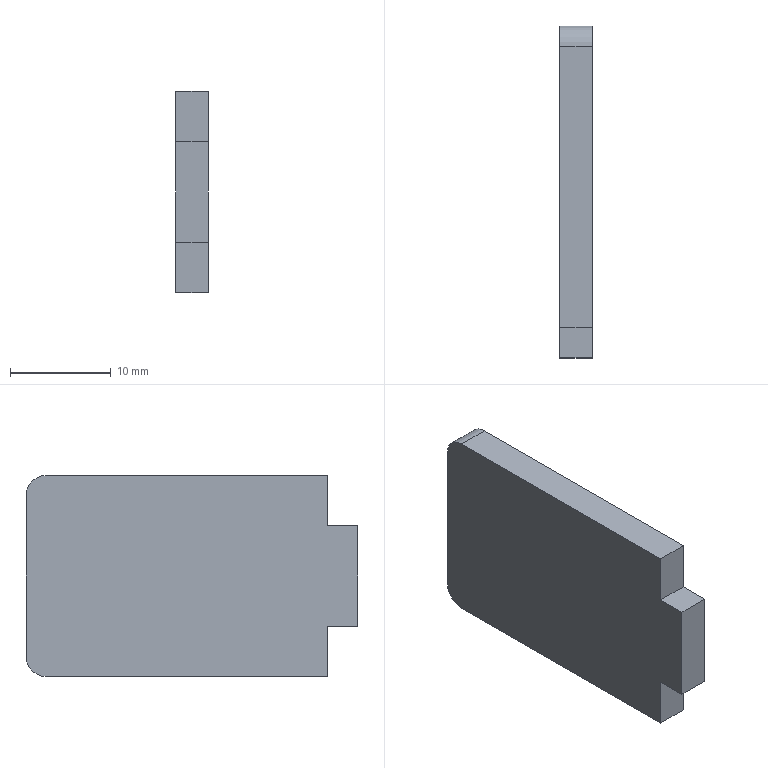Part | SolidWorks | features FlatPattern 1, SMBaseFlange 1, SheetMetal 1 | 1 solid | 12 faces | box 3.2 x 33 x 20 mm | volume 2011 mm3 | plane 10 | cylinder 2 | commonest cylinder face diameters 4 x2
STEP:
#1=CARTESIAN_POINT('',(0.,-30.,0.));
#2=VERTEX_POINT('',#1);
#3=CARTESIAN_POINT('',(0.,-30.,-5.));
#4=VERTEX_POINT('',#3);
#5=CARTESIAN_POINT('',(0.,-30.,0.));
#6=DIRECTION('',(0.,0.,-1.));
#7=VECTOR('',#6,1000.);
#8=LINE('',#5,#7);
#9=EDGE_CURVE('',#2,#4,#8,.T.);
#10=ORIENTED_EDGE('',*,*,#9,.F.);
#11=CARTESIAN_POINT('',(-3.2,-30.,0.));
#12=VERTEX_POINT('',#11);
#13=CARTESIAN_POINT('',(-3.2,-30.,0.));
#14=DIRECTION('',(1.,0.,0.));
#15=VECTOR('',#14,1000.);
#16=LINE('',#13,#15);
#17=EDGE_CURVE('',#12,#2,#16,.T.);
#18=ORIENTED_EDGE('',*,*,#17,.F.);
#19=CARTESIAN_POINT('',(-3.2,-30.,-5.));
#20=VERTEX_POINT('',#19);
#21=CARTESIAN_POINT('',(-3.2,-30.,0.));
#22=DIRECTION('',(0.,0.,-1.));
#23=VECTOR('',#22,1000.);
#24=LINE('',#21,#23);
#25=EDGE_CURVE('',#12,#20,#24,.T.);
#26=ORIENTED_EDGE('',*,*,#25,.T.);
#27=CARTESIAN_POINT('',(-3.2,-30.,-5.));
#28=DIRECTION('',(1.,0.,0.));
#29=VECTOR('',#28,1000.);
#30=LINE('',#27,#29);
#31=EDGE_CURVE('',#20,#4,#30,.T.);
#32=ORIENTED_EDGE('',*,*,#31,.T.);
#33=EDGE_LOOP('',(#10,#18,#26,#32));
#34=FACE_OUTER_BOUND('',#33,.T.);
#35=CARTESIAN_POINT('',(-3.2,-30.,0.));
#36=DIRECTION('',(0.,-1.,0.));
#37=DIRECTION('',(0.,0.,-1.));
#38=AXIS2_PLACEMENT_3D('',#35,#36,#37);
#39=PLANE('',#38);
#40=ADVANCED_FACE('',(#34),#39,.T.);
#41=CARTESIAN_POINT('',(0.,-2.,0.));
#42=VERTEX_POINT('',#41);
#43=CARTESIAN_POINT('',(0.,-2.,0.));
#44=DIRECTION('',(0.,-1.,0.));
#45=VECTOR('',#44,1000.);
#46=LINE('',#43,#45);
#47=EDGE_CURVE('',#42,#2,#46,.T.);
#48=ORIENTED_EDGE('',*,*,#47,.F.);
#49=CARTESIAN_POINT('',(-3.2,-2.,0.));
#50=VERTEX_POINT('',#49);
#51=CARTESIAN_POINT('',(-3.2,-2.,0.));
#52=DIRECTION('',(1.,0.,0.));
#53=VECTOR('',#52,1000.);
#54=LINE('',#51,#53);
#55=EDGE_CURVE('',#50,#42,#54,.T.);
#56=ORIENTED_EDGE('',*,*,#55,.F.);
#57=CARTESIAN_POINT('',(-3.2,-2.,0.));
#58=DIRECTION('',(0.,-1.,0.));
#59=VECTOR('',#58,1000.);
#60=LINE('',#57,#59);
#61=EDGE_CURVE('',#50,#12,#60,.T.);
#62=ORIENTED_EDGE('',*,*,#61,.T.);
#63=ORIENTED_EDGE('',*,*,#17,.T.);
#64=EDGE_LOOP('',(#48,#56,#62,#63));
#65=FACE_OUTER_BOUND('',#64,.T.);
#66=CARTESIAN_POINT('',(-3.2,-2.,0.));
#67=DIRECTION('',(0.,0.,1.));
#68=DIRECTION('',(1.,0.,0.));
#69=AXIS2_PLACEMENT_3D('',#66,#67,#68);
#70=PLANE('',#69);
#71=ADVANCED_FACE('',(#65),#70,.T.);
#72=CARTESIAN_POINT('',(0.,0.,-2.));
#73=VERTEX_POINT('',#72);
#74=CARTESIAN_POINT('',(0.,-2.,-2.));
#75=DIRECTION('',(1.,0.,0.));
#76=DIRECTION('',(0.,0.,1.));
#77=AXIS2_PLACEMENT_3D('',#74,#75,#76);
#78=CIRCLE('',#77,2.);
#79=EDGE_CURVE('',#73,#42,#78,.T.);
#80=ORIENTED_EDGE('',*,*,#79,.F.);
#81=CARTESIAN_POINT('',(-3.2,0.,-2.));
#82=VERTEX_POINT('',#81);
#83=CARTESIAN_POINT('',(-3.2,0.,-2.));
#84=DIRECTION('',(1.,0.,0.));
#85=VECTOR('',#84,1000.);
#86=LINE('',#83,#85);
#87=EDGE_CURVE('',#82,#73,#86,.T.);
#88=ORIENTED_EDGE('',*,*,#87,.F.);
#89=CARTESIAN_POINT('',(-3.2,-2.,-2.));
#90=DIRECTION('',(1.,0.,0.));
#91=DIRECTION('',(0.,0.,1.));
#92=AXIS2_PLACEMENT_3D('',#89,#90,#91);
#93=CIRCLE('',#92,2.);
#94=EDGE_CURVE('',#82,#50,#93,.T.);
#95=ORIENTED_EDGE('',*,*,#94,.T.);
#96=ORIENTED_EDGE('',*,*,#55,.T.);
#97=EDGE_LOOP('',(#80,#88,#95,#96));
#98=FACE_OUTER_BOUND('',#97,.T.);
#99=CARTESIAN_POINT('',(-3.2,-2.,-2.));
#100=DIRECTION('',(1.,0.,0.));
#101=DIRECTION('',(0.,0.,-1.));
#102=AXIS2_PLACEMENT_3D('',#99,#100,#101);
#103=CYLINDRICAL_SURFACE('',#102,2.);
#104=ADVANCED_FACE('',(#98),#103,.T.);
#105=CARTESIAN_POINT('',(0.,0.,-18.));
#106=VERTEX_POINT('',#105);
#107=CARTESIAN_POINT('',(0.,0.,-18.));
#108=DIRECTION('',(0.,0.,1.));
#109=VECTOR('',#108,1000.);
#110=LINE('',#107,#109);
#111=EDGE_CURVE('',#106,#73,#110,.T.);
#112=ORIENTED_EDGE('',*,*,#111,.F.);
#113=CARTESIAN_POINT('',(-3.2,0.,-18.));
#114=VERTEX_POINT('',#113);
#115=CARTESIAN_POINT('',(-3.2,0.,-18.));
#116=DIRECTION('',(1.,0.,0.));
#117=VECTOR('',#116,1000.);
#118=LINE('',#115,#117);
#119=EDGE_CURVE('',#114,#106,#118,.T.);
#120=ORIENTED_EDGE('',*,*,#119,.F.);
#121=CARTESIAN_POINT('',(-3.2,0.,-18.));
#122=DIRECTION('',(0.,0.,1.));
#123=VECTOR('',#122,1000.);
#124=LINE('',#121,#123);
#125=EDGE_CURVE('',#114,#82,#124,.T.);
#126=ORIENTED_EDGE('',*,*,#125,.T.);
#127=ORIENTED_EDGE('',*,*,#87,.T.);
#128=EDGE_LOOP('',(#112,#120,#126,#127));
#129=FACE_OUTER_BOUND('',#128,.T.);
#130=CARTESIAN_POINT('',(-3.2,0.,-18.));
#131=DIRECTION('',(0.,1.,0.));
#132=DIRECTION('',(0.,0.,1.));
#133=AXIS2_PLACEMENT_3D('',#130,#131,#132);
#134=PLANE('',#133);
#135=ADVANCED_FACE('',(#129),#134,.T.);
#136=CARTESIAN_POINT('',(0.,-2.,-20.));
#137=VERTEX_POINT('',#136);
#138=CARTESIAN_POINT('',(0.,-2.,-18.));
#139=DIRECTION('',(1.,0.,0.));
#140=DIRECTION('',(0.,0.,-1.));
#141=AXIS2_PLACEMENT_3D('',#138,#139,#140);
#142=CIRCLE('',#141,2.);
#143=EDGE_CURVE('',#137,#106,#142,.T.);
#144=ORIENTED_EDGE('',*,*,#143,.F.);
#145=CARTESIAN_POINT('',(-3.2,-2.,-20.));
#146=VERTEX_POINT('',#145);
#147=CARTESIAN_POINT('',(-3.2,-2.,-20.));
#148=DIRECTION('',(1.,0.,0.));
#149=VECTOR('',#148,1000.);
#150=LINE('',#147,#149);
#151=EDGE_CURVE('',#146,#137,#150,.T.);
#152=ORIENTED_EDGE('',*,*,#151,.F.);
#153=CARTESIAN_POINT('',(-3.2,-2.,-18.));
#154=DIRECTION('',(1.,0.,0.));
#155=DIRECTION('',(0.,0.,-1.));
#156=AXIS2_PLACEMENT_3D('',#153,#154,#155);
#157=CIRCLE('',#156,2.);
#158=EDGE_CURVE('',#146,#114,#157,.T.);
#159=ORIENTED_EDGE('',*,*,#158,.T.);
#160=ORIENTED_EDGE('',*,*,#119,.T.);
#161=EDGE_LOOP('',(#144,#152,#159,#160));
#162=FACE_OUTER_BOUND('',#161,.T.);
#163=CARTESIAN_POINT('',(-3.2,-2.,-18.));
#164=DIRECTION('',(1.,0.,0.));
#165=DIRECTION('',(0.,0.,-1.));
#166=AXIS2_PLACEMENT_3D('',#163,#164,#165);
#167=CYLINDRICAL_SURFACE('',#166,2.);
#168=ADVANCED_FACE('',(#162),#167,.T.);
#169=CARTESIAN_POINT('',(0.,-30.,-20.));
#170=VERTEX_POINT('',#169);
#171=CARTESIAN_POINT('',(0.,-30.,-20.));
#172=DIRECTION('',(0.,1.,0.));
#173=VECTOR('',#172,1000.);
#174=LINE('',#171,#173);
#175=EDGE_CURVE('',#170,#137,#174,.T.);
#176=ORIENTED_EDGE('',*,*,#175,.F.);
#177=CARTESIAN_POINT('',(-3.2,-30.,-20.));
#178=VERTEX_POINT('',#177);
#179=CARTESIAN_POINT('',(-3.2,-30.,-20.));
#180=DIRECTION('',(1.,0.,0.));
#181=VECTOR('',#180,1000.);
#182=LINE('',#179,#181);
#183=EDGE_CURVE('',#178,#170,#182,.T.);
#184=ORIENTED_EDGE('',*,*,#183,.F.);
#185=CARTESIAN_POINT('',(-3.2,-30.,-20.));
#186=DIRECTION('',(0.,1.,0.));
#187=VECTOR('',#186,1000.);
#188=LINE('',#185,#187);
#189=EDGE_CURVE('',#178,#146,#188,.T.);
#190=ORIENTED_EDGE('',*,*,#189,.T.);
#191=ORIENTED_EDGE('',*,*,#151,.T.);
#192=EDGE_LOOP('',(#176,#184,#190,#191));
#193=FACE_OUTER_BOUND('',#192,.T.);
#194=CARTESIAN_POINT('',(-3.2,-30.,-20.));
#195=DIRECTION('',(0.,0.,-1.));
#196=DIRECTION('',(-1.,0.,0.));
#197=AXIS2_PLACEMENT_3D('',#194,#195,#196);
#198=PLANE('',#197);
#199=ADVANCED_FACE('',(#193),#198,.T.);
#200=CARTESIAN_POINT('',(0.,-30.,-15.));
#201=VERTEX_POINT('',#200);
#202=CARTESIAN_POINT('',(0.,-30.,-15.));
#203=DIRECTION('',(0.,0.,-1.));
#204=VECTOR('',#203,1000.);
#205=LINE('',#202,#204);
#206=EDGE_CURVE('',#201,#170,#205,.T.);
#207=ORIENTED_EDGE('',*,*,#206,.F.);
#208=CARTESIAN_POINT('',(-3.2,-30.,-15.));
#209=VERTEX_POINT('',#208);
#210=CARTESIAN_POINT('',(-3.2,-30.,-15.));
#211=DIRECTION('',(1.,0.,0.));
#212=VECTOR('',#211,1000.);
#213=LINE('',#210,#212);
#214=EDGE_CURVE('',#209,#201,#213,.T.);
#215=ORIENTED_EDGE('',*,*,#214,.F.);
#216=CARTESIAN_POINT('',(-3.2,-30.,-15.));
#217=DIRECTION('',(0.,0.,-1.));
#218=VECTOR('',#217,1000.);
#219=LINE('',#216,#218);
#220=EDGE_CURVE('',#209,#178,#219,.T.);
#221=ORIENTED_EDGE('',*,*,#220,.T.);
#222=ORIENTED_EDGE('',*,*,#183,.T.);
#223=EDGE_LOOP('',(#207,#215,#221,#222));
#224=FACE_OUTER_BOUND('',#223,.T.);
#225=CARTESIAN_POINT('',(-3.2,-30.,-15.));
#226=DIRECTION('',(0.,-1.,0.));
#227=DIRECTION('',(0.,0.,-1.));
#228=AXIS2_PLACEMENT_3D('',#225,#226,#227);
#229=PLANE('',#228);
#230=ADVANCED_FACE('',(#224),#229,.T.);
#231=CARTESIAN_POINT('',(0.,-33.,-15.));
#232=VERTEX_POINT('',#231);
#233=CARTESIAN_POINT('',(0.,-33.,-15.));
#234=DIRECTION('',(0.,1.,0.));
#235=VECTOR('',#234,1000.);
#236=LINE('',#233,#235);
#237=EDGE_CURVE('',#232,#201,#236,.T.);
#238=ORIENTED_EDGE('',*,*,#237,.F.);
#239=CARTESIAN_POINT('',(-3.2,-33.,-15.));
#240=VERTEX_POINT('',#239);
#241=CARTESIAN_POINT('',(-3.2,-33.,-15.));
#242=DIRECTION('',(1.,0.,0.));
#243=VECTOR('',#242,1000.);
#244=LINE('',#241,#243);
#245=EDGE_CURVE('',#240,#232,#244,.T.);
#246=ORIENTED_EDGE('',*,*,#245,.F.);
#247=CARTESIAN_POINT('',(-3.2,-33.,-15.));
#248=DIRECTION('',(0.,1.,0.));
#249=VECTOR('',#248,1000.);
#250=LINE('',#247,#249);
#251=EDGE_CURVE('',#240,#209,#250,.T.);
#252=ORIENTED_EDGE('',*,*,#251,.T.);
#253=ORIENTED_EDGE('',*,*,#214,.T.);
#254=EDGE_LOOP('',(#238,#246,#252,#253));
#255=FACE_OUTER_BOUND('',#254,.T.);
#256=CARTESIAN_POINT('',(-3.2,-33.,-15.));
#257=DIRECTION('',(0.,0.,-1.));
#258=DIRECTION('',(-1.,0.,0.));
#259=AXIS2_PLACEMENT_3D('',#256,#257,#258);
#260=PLANE('',#259);
#261=ADVANCED_FACE('',(#255),#260,.T.);
#262=CARTESIAN_POINT('',(0.,-33.,-5.));
#263=VERTEX_POINT('',#262);
#264=CARTESIAN_POINT('',(0.,-33.,-5.));
#265=DIRECTION('',(0.,0.,-1.));
#266=VECTOR('',#265,1000.);
#267=LINE('',#264,#266);
#268=EDGE_CURVE('',#263,#232,#267,.T.);
#269=ORIENTED_EDGE('',*,*,#268,.F.);
#270=CARTESIAN_POINT('',(-3.2,-33.,-5.));
#271=VERTEX_POINT('',#270);
#272=CARTESIAN_POINT('',(-3.2,-33.,-5.));
#273=DIRECTION('',(1.,0.,0.));
#274=VECTOR('',#273,1000.);
#275=LINE('',#272,#274);
#276=EDGE_CURVE('',#271,#263,#275,.T.);
#277=ORIENTED_EDGE('',*,*,#276,.F.);
#278=CARTESIAN_POINT('',(-3.2,-33.,-5.));
#279=DIRECTION('',(0.,0.,-1.));
#280=VECTOR('',#279,1000.);
#281=LINE('',#278,#280);
#282=EDGE_CURVE('',#271,#240,#281,.T.);
#283=ORIENTED_EDGE('',*,*,#282,.T.);
#284=ORIENTED_EDGE('',*,*,#245,.T.);
#285=EDGE_LOOP('',(#269,#277,#283,#284));
#286=FACE_OUTER_BOUND('',#285,.T.);
#287=CARTESIAN_POINT('',(-3.2,-33.,-5.));
#288=DIRECTION('',(0.,-1.,0.));
#289=DIRECTION('',(0.,0.,-1.));
#290=AXIS2_PLACEMENT_3D('',#287,#288,#289);
#291=PLANE('',#290);
#292=ADVANCED_FACE('',(#286),#291,.T.);
#293=CARTESIAN_POINT('',(0.,-30.,-5.));
#294=DIRECTION('',(0.,-1.,0.));
#295=VECTOR('',#294,1000.);
#296=LINE('',#293,#295);
#297=EDGE_CURVE('',#4,#263,#296,.T.);
#298=ORIENTED_EDGE('',*,*,#297,.F.);
#299=ORIENTED_EDGE('',*,*,#31,.F.);
#300=CARTESIAN_POINT('',(-3.2,-30.,-5.));
#301=DIRECTION('',(0.,-1.,0.));
#302=VECTOR('',#301,1000.);
#303=LINE('',#300,#302);
#304=EDGE_CURVE('',#20,#271,#303,.T.);
#305=ORIENTED_EDGE('',*,*,#304,.T.);
#306=ORIENTED_EDGE('',*,*,#276,.T.);
#307=EDGE_LOOP('',(#298,#299,#305,#306));
#308=FACE_OUTER_BOUND('',#307,.T.);
#309=CARTESIAN_POINT('',(-3.2,-30.,-5.));
#310=DIRECTION('',(0.,0.,1.));
#311=DIRECTION('',(1.,0.,0.));
#312=AXIS2_PLACEMENT_3D('',#309,#310,#311);
#313=PLANE('',#312);
#314=ADVANCED_FACE('',(#308),#313,.T.);
#315=ORIENTED_EDGE('',*,*,#25,.F.);
#316=ORIENTED_EDGE('',*,*,#61,.F.);
#317=ORIENTED_EDGE('',*,*,#94,.F.);
#318=ORIENTED_EDGE('',*,*,#125,.F.);
#319=ORIENTED_EDGE('',*,*,#158,.F.);
#320=ORIENTED_EDGE('',*,*,#189,.F.);
#321=ORIENTED_EDGE('',*,*,#220,.F.);
#322=ORIENTED_EDGE('',*,*,#251,.F.);
#323=ORIENTED_EDGE('',*,*,#282,.F.);
#324=ORIENTED_EDGE('',*,*,#304,.F.);
#325=EDGE_LOOP('',(#315,#316,#317,#318,#319,#320,#321,#322,#323,#324));
#326=FACE_OUTER_BOUND('',#325,.T.);
#327=CARTESIAN_POINT('',(-3.2,-2.,-18.));
#328=DIRECTION('',(1.,0.,0.));
#329=DIRECTION('',(0.,0.,-1.));
#330=AXIS2_PLACEMENT_3D('',#327,#328,#329);
#331=PLANE('',#330);
#332=ADVANCED_FACE('',(#326),#331,.F.);
#333=ORIENTED_EDGE('',*,*,#9,.T.);
#334=ORIENTED_EDGE('',*,*,#297,.T.);
#335=ORIENTED_EDGE('',*,*,#268,.T.);
#336=ORIENTED_EDGE('',*,*,#237,.T.);
#337=ORIENTED_EDGE('',*,*,#206,.T.);
#338=ORIENTED_EDGE('',*,*,#175,.T.);
#339=ORIENTED_EDGE('',*,*,#143,.T.);
#340=ORIENTED_EDGE('',*,*,#111,.T.);
#341=ORIENTED_EDGE('',*,*,#79,.T.);
#342=ORIENTED_EDGE('',*,*,#47,.T.);
#343=EDGE_LOOP('',(#333,#334,#335,#336,#337,#338,#339,#340,#341,#342));
#344=FACE_OUTER_BOUND('',#343,.T.);
#345=CARTESIAN_POINT('',(0.,-2.,-18.));
#346=DIRECTION('',(1.,0.,0.));
#347=DIRECTION('',(0.,0.,-1.));
#348=AXIS2_PLACEMENT_3D('',#345,#346,#347);
#349=PLANE('',#348);
#350=ADVANCED_FACE('',(#344),#349,.T.);
#351=CLOSED_SHELL('',(#40,#71,#104,#135,#168,#199,#230,#261,#292,#314,#332,#350));
#352=MANIFOLD_SOLID_BREP('',#351);
#353=CARTESIAN_POINT('',(0.,0.,0.));
#354=DIRECTION('',(0.,0.,1.));
#355=DIRECTION('',(1.,0.,0.));
#356=AXIS2_PLACEMENT_3D('',#353,#354,#355);
#357=(LENGTH_UNIT()NAMED_UNIT(*)SI_UNIT(.MILLI.,.METRE.));
#358=UNCERTAINTY_MEASURE_WITH_UNIT(LENGTH_MEASURE(0.00001),#357,'','');
#359=(NAMED_UNIT(*)PLANE_ANGLE_UNIT()SI_UNIT($,.RADIAN.));
#360=(NAMED_UNIT(*)SI_UNIT($,.STERADIAN.)SOLID_ANGLE_UNIT());
#361=(GEOMETRIC_REPRESENTATION_CONTEXT(3)GLOBAL_UNCERTAINTY_ASSIGNED_CONTEXT((#358))GLOBAL_UNIT_ASSIGNED_CONTEXT((#357,#359,#360))REPRESENTATION_CONTEXT('',''));
#362=ADVANCED_BREP_SHAPE_REPRESENTATION('',(#352,#356),#361);